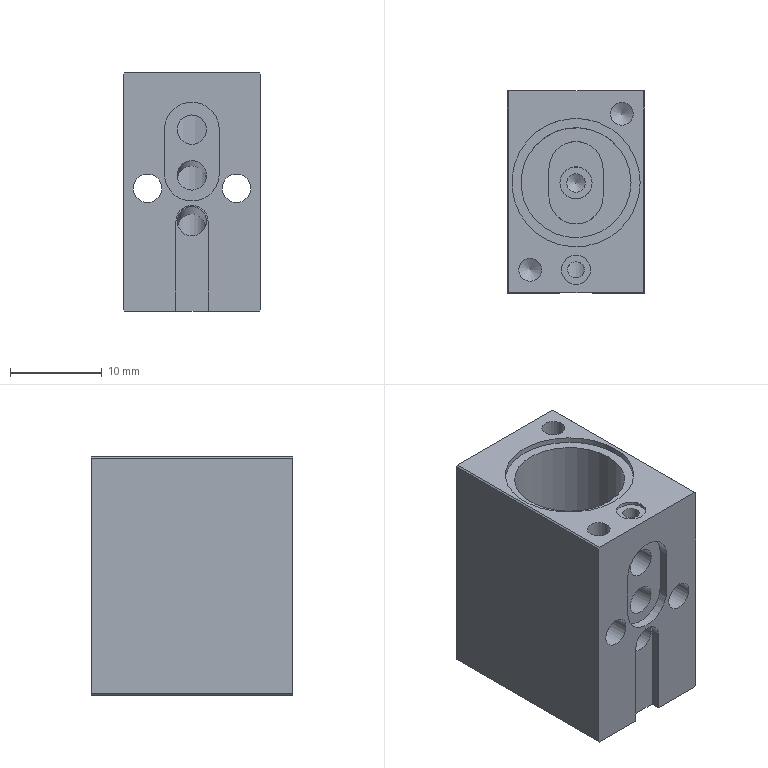NC program | NX | posted with a generic post | part box 15 x 22 x 26 mm
Lines 5152 to 5185 of 5185:
(DRILLING_3 , TOOL : D1.8钻头)
N10218 T07 M6
N10220 G54
N10222 G17 G0 G90 X0. Y12. B0. C0. S3000 M3
N10224 G43 Z30. H7
N10226 G94 G81 G99 Z-24.7 F120. R-10.7
N10228 G80
N10230 G0 X0. Y12. Z30.
N10232 M5
(DRILLING_3_COPY , TOOL : D2.8钻头)
N10234 T15 M6
N10236 G54
N10238 G17 G0 G90 X0. Y12. B0. C0. S3000 M3
N10240 G43 Z30. H15
N10242 G94 G81 G99 Z-21.2 F120. R-10.7
N10244 G80
N10246 G0 X0. Y12. Z30.
N10248 M5
(DRILLING_3_COPY_1 , TOOL : 成型刀)
N10250 T16 M6
N10252 G54
N10254 G17 G0 G90 X0. Y12. B0. C0. S3000 M3
N10256 G43 Z30. H16
N10258 G94 G81 G99 Z-24.85 F40. R-10.7
N10260 G80
N10262 G0 X0. Y12. Z30.
N10264 M5
N10266 M2